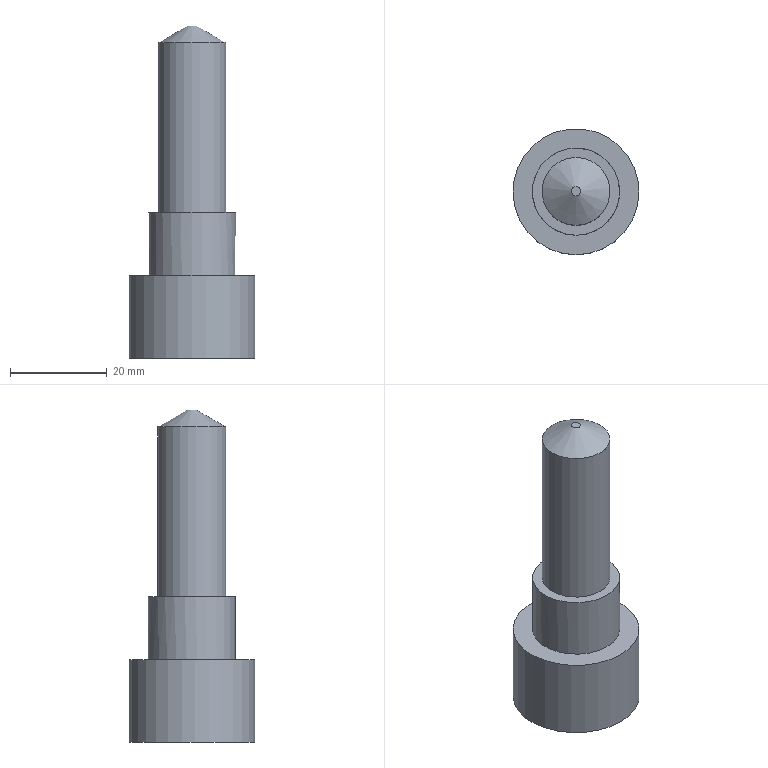Part | STEP file | solid 205 | 1 solid | 8 faces | box 26 x 26 x 68.5 mm | volume 17929 mm3 | plane 4 | cylinder 3 | cone 1 | commonest cylinder face diameters 14 x1 18 x1 26 x1